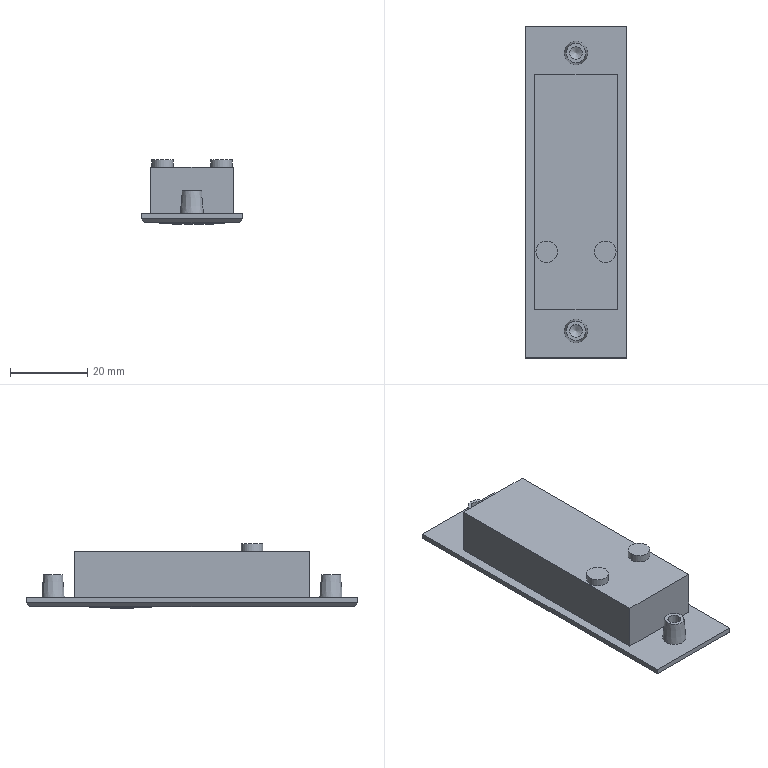Part | STEP file | door lock catch | 1 solid | 132 faces | box 26.4 x 86 x 16.7 mm | volume 21050 mm3 | plane 84 | spline 40 | cylinder 4 | cone 4 | commonest cylinder face diameters 3.3 x2 5.6 x2